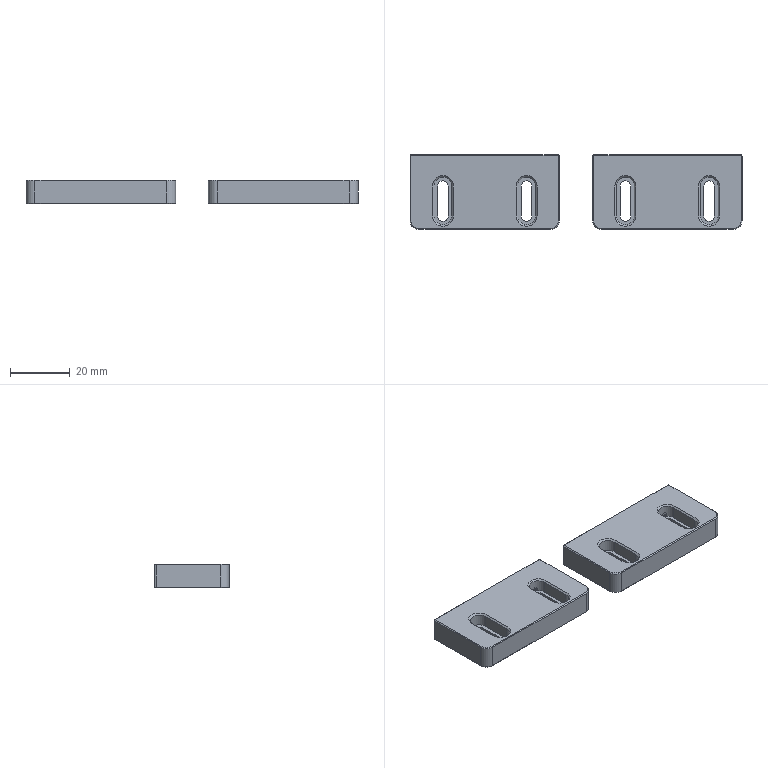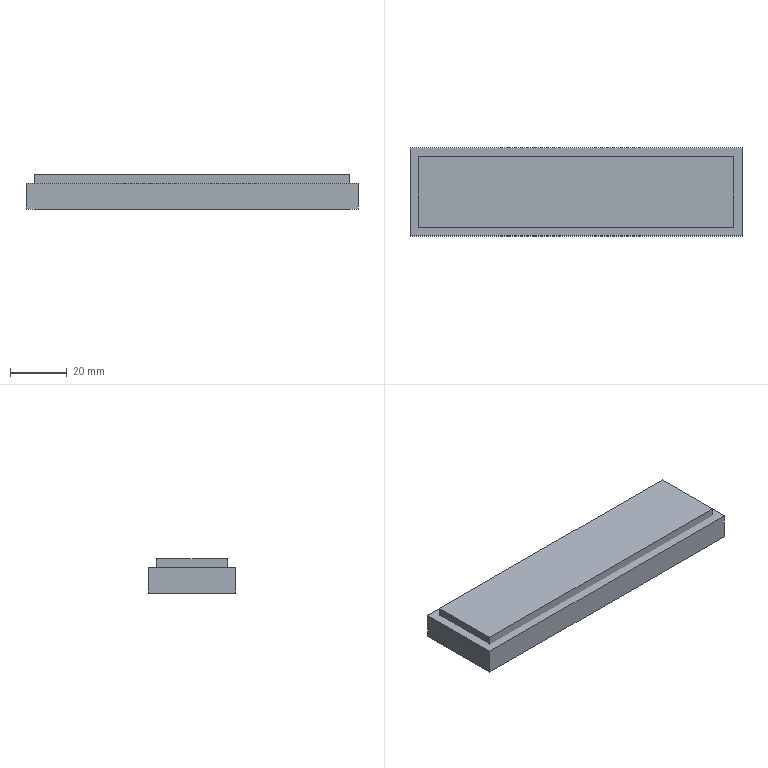CAM job | NX | 3-axis milling | part box 111 x 25 x 8 mm | stock box 117 x 31 x 12 mm
Tools:
number,name,description,diameter,corner_radius,flute_length,length,flutes
1,D63,Milling Tool-5 Parameters,63.0,0.0,50.0,75.0,2
2,D4A45,Milling Tool-5 Parameters,4.0,0.0,2.0,2.0,2
6,D6,Milling Tool-5 Parameters,6.0,0.0,50.0,75.0,2
4,D4,Milling Tool-5 Parameters,4.0,0.0,50.0,75.0,2
3,D3,Milling Tool-5 Parameters,3.0,0.0,50.0,75.0,2
Operations:
program,operation,operation_type,tool,method,geometry_group,spindle_rpm,surface_speed,feed_per_tooth,feed_cut,feed_plunge,cut_length_mm,path_length_mm,cut_time_min,machine_time_min
1虎钳,FLOOR_WALL,VolumeBased25DMillingOperation,D63,METHOD,A,6500.0,1286.0,0.0962,1250.0,100.0,192.0,246.0,0.1536,0.159
1虎钳,ZLEVEL_PROFILE_1_COPY_1_COPY_COPY,ZLevelMilling,D4A45,METHOD,A,9500.0,179.0,0.0526,1000.0,100.0,472.155,1045.896,0.4722,0.5295
1虎钳,ZLEVEL_PROFILE_COPY_COPY_1_COPY,ZLevelMilling,D6,METHOD,A,9500.0,179.0,0.1158,2200.0,1000.0,5463.965,5711.234,2.525,2.55
1虎钳,ZLEVEL_PROFILE_COPY_COPY_1_COPY_COPY,ZLevelMilling,D4,METHOD,A,9500.0,179.0,0.0868,1650.0,1000.0,1181.214,1520.813,0.7761,0.8101
1虎钳,ZLEVEL_PROFILE_COPY_COPY_1_COPY_COPY_COPY,ZLevelMilling,D3,METHOD,A,9500.0,89.0,0.0684,1300.0,1000.0,1731.852,2099.358,1.362,1.399
1虎钳,ZLEVEL_PROFILE_COPY_COPY_COPY_COPY_COPY,ZLevelMilling,D4,MILL_FINISH,A,9500.0,119.0,0.0632,1200.0,1000.0,327.199,534.991,0.2733,0.2941
2,FLOOR_WALL_COPY,VolumeBased25DMillingOperation,D63,METHOD,B,6500.0,1286.0,0.0962,1250.0,100.0,744.0,1488.001,0.5952,0.6696
2,ZLEVEL_PROFILE_1_COPY_1_COPY_COPY_COPY,ZLevelMilling,D4A45,METHOD,B,9500.0,179.0,0.0526,1000.0,100.0,424.038,1011.633,0.424,0.4828